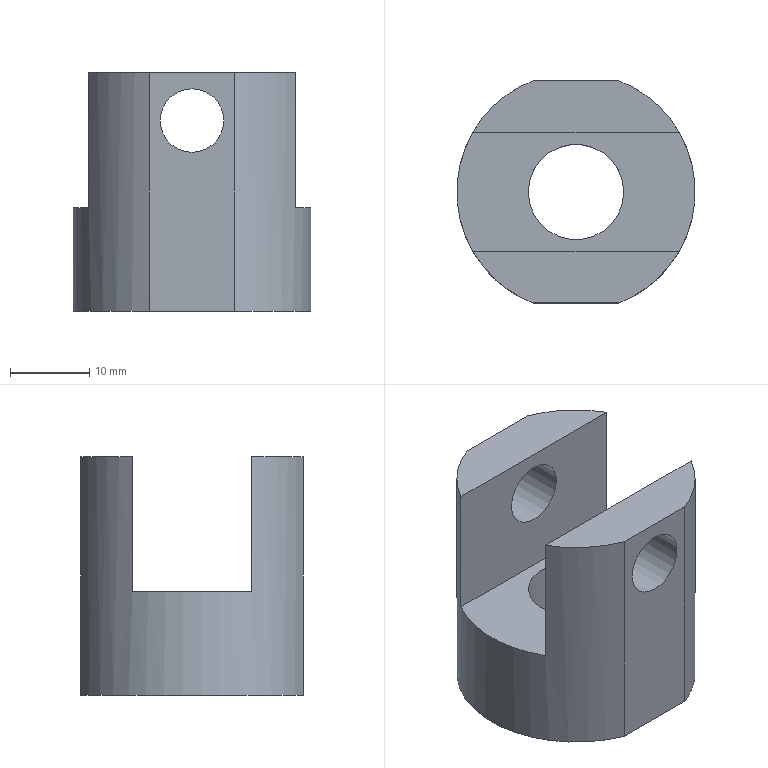Part | NX | features pneumatic support1 2 | 1 solid | 13 faces | box 30 x 28 x 30 mm | volume 11330 mm3 | plane 8 | cylinder 5 | commonest cylinder face diameters 8 x2 30 x2 12 x1
STEP:
#1=CARTESIAN_POINT('',(0.,-7.5,28.));
#2=VERTEX_POINT('',#1);
#3=CARTESIAN_POINT('',(0.,-7.5,24.));
#4=DIRECTION('',(0.,1.,0.));
#5=DIRECTION('',(0.,0.,1.));
#6=AXIS2_PLACEMENT_3D('',#3,#4,#5);
#7=CIRCLE('',#6,4.);
#8=EDGE_CURVE('',#2,#2,#7,.T.);
#9=ORIENTED_EDGE('',*,*,#8,.T.);
#10=EDGE_LOOP('',(#9));
#11=FACE_BOUND('',#10,.T.);
#12=CARTESIAN_POINT('',(0.,-14.,28.));
#13=VERTEX_POINT('',#12);
#14=CARTESIAN_POINT('',(0.,-14.,24.));
#15=DIRECTION('',(0.,1.,0.));
#16=DIRECTION('',(0.,0.,1.));
#17=AXIS2_PLACEMENT_3D('',#14,#15,#16);
#18=CIRCLE('',#17,4.);
#19=EDGE_CURVE('',#13,#13,#18,.T.);
#20=ORIENTED_EDGE('',*,*,#19,.F.);
#21=EDGE_LOOP('',(#20));
#22=FACE_BOUND('',#21,.T.);
#23=CARTESIAN_POINT('',(0.,-20.,24.));
#24=DIRECTION('',(0.,1.,0.));
#25=DIRECTION('',(0.,0.,1.));
#26=AXIS2_PLACEMENT_3D('',#23,#24,#25);
#27=CYLINDRICAL_SURFACE('',#26,4.);
#28=ADVANCED_FACE('',(#11,#22),#27,.F.);
#29=CARTESIAN_POINT('',(-6.,0.,13.));
#30=VERTEX_POINT('',#29);
#31=CARTESIAN_POINT('',(0.,0.,13.));
#32=DIRECTION('',(0.,0.,-1.));
#33=DIRECTION('',(-1.,0.,0.));
#34=AXIS2_PLACEMENT_3D('',#31,#32,#33);
#35=CIRCLE('',#34,6.);
#36=EDGE_CURVE('',#30,#30,#35,.T.);
#37=ORIENTED_EDGE('',*,*,#36,.F.);
#38=EDGE_LOOP('',(#37));
#39=FACE_BOUND('',#38,.T.);
#40=CARTESIAN_POINT('',(-6.,0.,0.));
#41=VERTEX_POINT('',#40);
#42=CARTESIAN_POINT('',(0.,0.,0.));
#43=DIRECTION('',(0.,0.,-1.));
#44=DIRECTION('',(-1.,0.,0.));
#45=AXIS2_PLACEMENT_3D('',#42,#43,#44);
#46=CIRCLE('',#45,6.);
#47=EDGE_CURVE('',#41,#41,#46,.T.);
#48=ORIENTED_EDGE('',*,*,#47,.T.);
#49=EDGE_LOOP('',(#48));
#50=FACE_BOUND('',#49,.T.);
#51=CARTESIAN_POINT('',(0.,0.,0.));
#52=DIRECTION('',(0.,0.,-1.));
#53=DIRECTION('',(-1.,0.,0.));
#54=AXIS2_PLACEMENT_3D('',#51,#52,#53);
#55=CYLINDRICAL_SURFACE('',#54,6.);
#56=ADVANCED_FACE('',(#39,#50),#55,.F.);
#57=CARTESIAN_POINT('',(0.,7.5,28.));
#58=VERTEX_POINT('',#57);
#59=CARTESIAN_POINT('',(0.,7.5,24.));
#60=DIRECTION('',(0.,1.,0.));
#61=DIRECTION('',(0.,0.,1.));
#62=AXIS2_PLACEMENT_3D('',#59,#60,#61);
#63=CIRCLE('',#62,4.);
#64=EDGE_CURVE('',#58,#58,#63,.F.);
#65=ORIENTED_EDGE('',*,*,#64,.T.);
#66=EDGE_LOOP('',(#65));
#67=FACE_BOUND('',#66,.T.);
#68=CARTESIAN_POINT('',(0.,14.,28.));
#69=VERTEX_POINT('',#68);
#70=CARTESIAN_POINT('',(0.,14.,24.));
#71=DIRECTION('',(0.,1.,0.));
#72=DIRECTION('',(0.,0.,1.));
#73=AXIS2_PLACEMENT_3D('',#70,#71,#72);
#74=CIRCLE('',#73,4.);
#75=EDGE_CURVE('',#69,#69,#74,.F.);
#76=ORIENTED_EDGE('',*,*,#75,.F.);
#77=EDGE_LOOP('',(#76));
#78=FACE_BOUND('',#77,.T.);
#79=CARTESIAN_POINT('',(0.,-20.,24.));
#80=DIRECTION('',(0.,1.,0.));
#81=DIRECTION('',(0.,0.,1.));
#82=AXIS2_PLACEMENT_3D('',#79,#80,#81);
#83=CYLINDRICAL_SURFACE('',#82,4.);
#84=ADVANCED_FACE('',(#67,#78),#83,.F.);
#85=CARTESIAN_POINT('',(-5.385,14.,0.));
#86=VERTEX_POINT('',#85);
#87=CARTESIAN_POINT('',(-5.385,14.,30.));
#88=VERTEX_POINT('',#87);
#89=CARTESIAN_POINT('',(-5.385,14.,30.));
#90=DIRECTION('',(0.,0.,1.));
#91=VECTOR('',#90,1000.);
#92=LINE('',#89,#91);
#93=EDGE_CURVE('',#86,#88,#92,.T.);
#94=ORIENTED_EDGE('',*,*,#93,.F.);
#95=CARTESIAN_POINT('',(-5.385,-14.,0.));
#96=VERTEX_POINT('',#95);
#97=CARTESIAN_POINT('',(0.,0.,0.));
#98=DIRECTION('',(0.,0.,-1.));
#99=DIRECTION('',(-1.,0.,0.));
#100=AXIS2_PLACEMENT_3D('',#97,#98,#99);
#101=CIRCLE('',#100,15.);
#102=EDGE_CURVE('',#86,#96,#101,.F.);
#103=ORIENTED_EDGE('',*,*,#102,.T.);
#104=CARTESIAN_POINT('',(-5.385,-14.,30.));
#105=VERTEX_POINT('',#104);
#106=CARTESIAN_POINT('',(-5.385,-14.,30.));
#107=DIRECTION('',(0.,0.,-1.));
#108=VECTOR('',#107,1000.);
#109=LINE('',#106,#108);
#110=EDGE_CURVE('',#105,#96,#109,.T.);
#111=ORIENTED_EDGE('',*,*,#110,.F.);
#112=CARTESIAN_POINT('',(-12.99,-7.5,30.));
#113=VERTEX_POINT('',#112);
#114=CARTESIAN_POINT('',(0.,0.,30.));
#115=DIRECTION('',(0.,0.,-1.));
#116=DIRECTION('',(-1.,0.,0.));
#117=AXIS2_PLACEMENT_3D('',#114,#115,#116);
#118=CIRCLE('',#117,15.);
#119=EDGE_CURVE('',#113,#105,#118,.F.);
#120=ORIENTED_EDGE('',*,*,#119,.F.);
#121=CARTESIAN_POINT('',(-12.99,-7.5,13.));
#122=VERTEX_POINT('',#121);
#123=CARTESIAN_POINT('',(-12.99,-7.5,13.));
#124=DIRECTION('',(0.,0.,-1.));
#125=VECTOR('',#124,1000.);
#126=LINE('',#123,#125);
#127=EDGE_CURVE('',#113,#122,#126,.T.);
#128=ORIENTED_EDGE('',*,*,#127,.T.);
#129=CARTESIAN_POINT('',(-12.99,7.5,13.));
#130=VERTEX_POINT('',#129);
#131=CARTESIAN_POINT('',(0.,0.,13.));
#132=DIRECTION('',(0.,0.,-1.));
#133=DIRECTION('',(-1.,0.,0.));
#134=AXIS2_PLACEMENT_3D('',#131,#132,#133);
#135=CIRCLE('',#134,15.);
#136=EDGE_CURVE('',#130,#122,#135,.F.);
#137=ORIENTED_EDGE('',*,*,#136,.F.);
#138=CARTESIAN_POINT('',(-12.99,7.5,30.));
#139=VERTEX_POINT('',#138);
#140=CARTESIAN_POINT('',(-12.99,7.5,13.));
#141=DIRECTION('',(0.,0.,1.));
#142=VECTOR('',#141,1000.);
#143=LINE('',#140,#142);
#144=EDGE_CURVE('',#130,#139,#143,.T.);
#145=ORIENTED_EDGE('',*,*,#144,.T.);
#146=CARTESIAN_POINT('',(0.,0.,30.));
#147=DIRECTION('',(0.,0.,-1.));
#148=DIRECTION('',(-1.,0.,0.));
#149=AXIS2_PLACEMENT_3D('',#146,#147,#148);
#150=CIRCLE('',#149,15.);
#151=EDGE_CURVE('',#88,#139,#150,.F.);
#152=ORIENTED_EDGE('',*,*,#151,.F.);
#153=EDGE_LOOP('',(#94,#103,#111,#120,#128,#137,#145,#152));
#154=FACE_BOUND('',#153,.T.);
#155=CARTESIAN_POINT('',(0.,0.,30.));
#156=DIRECTION('',(0.,0.,-1.));
#157=DIRECTION('',(-1.,0.,0.));
#158=AXIS2_PLACEMENT_3D('',#155,#156,#157);
#159=CYLINDRICAL_SURFACE('',#158,15.);
#160=ADVANCED_FACE('',(#154),#159,.T.);
#161=ORIENTED_EDGE('',*,*,#144,.F.);
#162=CARTESIAN_POINT('',(12.99,7.5,13.));
#163=VERTEX_POINT('',#162);
#164=CARTESIAN_POINT('',(-15.,7.5,13.));
#165=DIRECTION('',(1.,0.,0.));
#166=VECTOR('',#165,1000.);
#167=LINE('',#164,#166);
#168=EDGE_CURVE('',#163,#130,#167,.F.);
#169=ORIENTED_EDGE('',*,*,#168,.F.);
#170=CARTESIAN_POINT('',(12.99,7.5,30.));
#171=VERTEX_POINT('',#170);
#172=CARTESIAN_POINT('',(12.99,7.5,30.));
#173=DIRECTION('',(0.,0.,-1.));
#174=VECTOR('',#173,1000.);
#175=LINE('',#172,#174);
#176=EDGE_CURVE('',#171,#163,#175,.T.);
#177=ORIENTED_EDGE('',*,*,#176,.F.);
#178=CARTESIAN_POINT('',(0.,7.5,30.));
#179=DIRECTION('',(1.,0.,0.));
#180=VECTOR('',#179,1000.);
#181=LINE('',#178,#180);
#182=EDGE_CURVE('',#139,#171,#181,.T.);
#183=ORIENTED_EDGE('',*,*,#182,.F.);
#184=EDGE_LOOP('',(#161,#169,#177,#183));
#185=FACE_BOUND('',#184,.T.);
#186=ORIENTED_EDGE('',*,*,#64,.F.);
#187=EDGE_LOOP('',(#186));
#188=FACE_BOUND('',#187,.T.);
#189=CARTESIAN_POINT('',(15.,7.5,13.));
#190=DIRECTION('',(0.,1.,0.));
#191=DIRECTION('',(0.,0.,1.));
#192=AXIS2_PLACEMENT_3D('',#189,#190,#191);
#193=PLANE('',#192);
#194=ADVANCED_FACE('',(#185,#188),#193,.F.);
#195=CARTESIAN_POINT('',(12.99,-7.5,13.));
#196=VERTEX_POINT('',#195);
#197=CARTESIAN_POINT('',(15.,-7.5,13.));
#198=DIRECTION('',(1.,0.,0.));
#199=VECTOR('',#198,1000.);
#200=LINE('',#197,#199);
#201=EDGE_CURVE('',#122,#196,#200,.T.);
#202=ORIENTED_EDGE('',*,*,#201,.T.);
#203=CARTESIAN_POINT('',(0.,0.,13.));
#204=DIRECTION('',(0.,0.,-1.));
#205=DIRECTION('',(-1.,0.,0.));
#206=AXIS2_PLACEMENT_3D('',#203,#204,#205);
#207=CIRCLE('',#206,15.);
#208=EDGE_CURVE('',#163,#196,#207,.T.);
#209=ORIENTED_EDGE('',*,*,#208,.F.);
#210=ORIENTED_EDGE('',*,*,#168,.T.);
#211=ORIENTED_EDGE('',*,*,#136,.T.);
#212=EDGE_LOOP('',(#202,#209,#210,#211));
#213=FACE_BOUND('',#212,.T.);
#214=ORIENTED_EDGE('',*,*,#36,.T.);
#215=EDGE_LOOP('',(#214));
#216=FACE_BOUND('',#215,.T.);
#217=CARTESIAN_POINT('',(-15.,7.5,13.));
#218=DIRECTION('',(0.,0.,1.));
#219=DIRECTION('',(1.,0.,0.));
#220=AXIS2_PLACEMENT_3D('',#217,#218,#219);
#221=PLANE('',#220);
#222=ADVANCED_FACE('',(#213,#216),#221,.T.);
#223=CARTESIAN_POINT('',(12.99,-7.5,30.));
#224=VERTEX_POINT('',#223);
#225=CARTESIAN_POINT('',(12.99,-7.5,30.));
#226=DIRECTION('',(0.,0.,-1.));
#227=VECTOR('',#226,1000.);
#228=LINE('',#225,#227);
#229=EDGE_CURVE('',#196,#224,#228,.F.);
#230=ORIENTED_EDGE('',*,*,#229,.F.);
#231=ORIENTED_EDGE('',*,*,#201,.F.);
#232=ORIENTED_EDGE('',*,*,#127,.F.);
#233=CARTESIAN_POINT('',(0.,-7.5,30.));
#234=DIRECTION('',(1.,0.,0.));
#235=VECTOR('',#234,1000.);
#236=LINE('',#233,#235);
#237=EDGE_CURVE('',#224,#113,#236,.F.);
#238=ORIENTED_EDGE('',*,*,#237,.F.);
#239=EDGE_LOOP('',(#230,#231,#232,#238));
#240=FACE_BOUND('',#239,.T.);
#241=ORIENTED_EDGE('',*,*,#8,.F.);
#242=EDGE_LOOP('',(#241));
#243=FACE_BOUND('',#242,.T.);
#244=CARTESIAN_POINT('',(15.,-7.5,13.));
#245=DIRECTION('',(0.,-1.,0.));
#246=DIRECTION('',(0.,0.,-1.));
#247=AXIS2_PLACEMENT_3D('',#244,#245,#246);
#248=PLANE('',#247);
#249=ADVANCED_FACE('',(#240,#243),#248,.F.);
#250=CARTESIAN_POINT('',(5.385,-14.,30.));
#251=VERTEX_POINT('',#250);
#252=CARTESIAN_POINT('',(0.,0.,30.));
#253=DIRECTION('',(0.,0.,-1.));
#254=DIRECTION('',(-1.,0.,0.));
#255=AXIS2_PLACEMENT_3D('',#252,#253,#254);
#256=CIRCLE('',#255,15.);
#257=EDGE_CURVE('',#224,#251,#256,.T.);
#258=ORIENTED_EDGE('',*,*,#257,.F.);
#259=ORIENTED_EDGE('',*,*,#237,.T.);
#260=ORIENTED_EDGE('',*,*,#119,.T.);
#261=CARTESIAN_POINT('',(15.,-14.,30.));
#262=DIRECTION('',(1.,0.,0.));
#263=VECTOR('',#262,1000.);
#264=LINE('',#261,#263);
#265=EDGE_CURVE('',#251,#105,#264,.F.);
#266=ORIENTED_EDGE('',*,*,#265,.F.);
#267=EDGE_LOOP('',(#258,#259,#260,#266));
#268=FACE_BOUND('',#267,.T.);
#269=CARTESIAN_POINT('',(0.,0.,30.));
#270=DIRECTION('',(0.,0.,1.));
#271=DIRECTION('',(1.,0.,0.));
#272=AXIS2_PLACEMENT_3D('',#269,#270,#271);
#273=PLANE('',#272);
#274=ADVANCED_FACE('',(#268),#273,.T.);
#275=CARTESIAN_POINT('',(5.385,-14.,0.));
#276=VERTEX_POINT('',#275);
#277=CARTESIAN_POINT('',(5.385,-14.,30.));
#278=DIRECTION('',(0.,0.,-1.));
#279=VECTOR('',#278,1000.);
#280=LINE('',#277,#279);
#281=EDGE_CURVE('',#251,#276,#280,.T.);
#282=ORIENTED_EDGE('',*,*,#281,.F.);
#283=ORIENTED_EDGE('',*,*,#265,.T.);
#284=ORIENTED_EDGE('',*,*,#110,.T.);
#285=CARTESIAN_POINT('',(0.,-14.,0.));
#286=DIRECTION('',(1.,0.,0.));
#287=VECTOR('',#286,1000.);
#288=LINE('',#285,#287);
#289=EDGE_CURVE('',#96,#276,#288,.T.);
#290=ORIENTED_EDGE('',*,*,#289,.T.);
#291=EDGE_LOOP('',(#282,#283,#284,#290));
#292=FACE_BOUND('',#291,.T.);
#293=ORIENTED_EDGE('',*,*,#19,.T.);
#294=EDGE_LOOP('',(#293));
#295=FACE_BOUND('',#294,.T.);
#296=CARTESIAN_POINT('',(15.,-14.,30.));
#297=DIRECTION('',(0.,-1.,0.));
#298=DIRECTION('',(0.,0.,-1.));
#299=AXIS2_PLACEMENT_3D('',#296,#297,#298);
#300=PLANE('',#299);
#301=ADVANCED_FACE('',(#292,#295),#300,.T.);
#302=ORIENTED_EDGE('',*,*,#102,.F.);
#303=CARTESIAN_POINT('',(5.385,14.,0.));
#304=VERTEX_POINT('',#303);
#305=CARTESIAN_POINT('',(15.,14.,0.));
#306=DIRECTION('',(1.,0.,0.));
#307=VECTOR('',#306,1000.);
#308=LINE('',#305,#307);
#309=EDGE_CURVE('',#304,#86,#308,.F.);
#310=ORIENTED_EDGE('',*,*,#309,.F.);
#311=CARTESIAN_POINT('',(0.,0.,0.));
#312=DIRECTION('',(0.,0.,-1.));
#313=DIRECTION('',(-1.,0.,0.));
#314=AXIS2_PLACEMENT_3D('',#311,#312,#313);
#315=CIRCLE('',#314,15.);
#316=EDGE_CURVE('',#276,#304,#315,.F.);
#317=ORIENTED_EDGE('',*,*,#316,.F.);
#318=ORIENTED_EDGE('',*,*,#289,.F.);
#319=EDGE_LOOP('',(#302,#310,#317,#318));
#320=FACE_BOUND('',#319,.T.);
#321=ORIENTED_EDGE('',*,*,#47,.F.);
#322=EDGE_LOOP('',(#321));
#323=FACE_BOUND('',#322,.T.);
#324=CARTESIAN_POINT('',(0.,0.,0.));
#325=DIRECTION('',(0.,0.,1.));
#326=DIRECTION('',(1.,0.,0.));
#327=AXIS2_PLACEMENT_3D('',#324,#325,#326);
#328=PLANE('',#327);
#329=ADVANCED_FACE('',(#320,#323),#328,.F.);
#330=ORIENTED_EDGE('',*,*,#93,.T.);
#331=CARTESIAN_POINT('',(5.385,14.,30.));
#332=VERTEX_POINT('',#331);
#333=CARTESIAN_POINT('',(0.,14.,30.));
#334=DIRECTION('',(1.,0.,0.));
#335=VECTOR('',#334,1000.);
#336=LINE('',#333,#335);
#337=EDGE_CURVE('',#332,#88,#336,.F.);
#338=ORIENTED_EDGE('',*,*,#337,.F.);
#339=CARTESIAN_POINT('',(5.385,14.,30.));
#340=DIRECTION('',(0.,0.,-1.));
#341=VECTOR('',#340,1000.);
#342=LINE('',#339,#341);
#343=EDGE_CURVE('',#304,#332,#342,.F.);
#344=ORIENTED_EDGE('',*,*,#343,.F.);
#345=ORIENTED_EDGE('',*,*,#309,.T.);
#346=EDGE_LOOP('',(#330,#338,#344,#345));
#347=FACE_BOUND('',#346,.T.);
#348=ORIENTED_EDGE('',*,*,#75,.T.);
#349=EDGE_LOOP('',(#348));
#350=FACE_BOUND('',#349,.T.);
#351=CARTESIAN_POINT('',(15.,14.,30.));
#352=DIRECTION('',(0.,1.,0.));
#353=DIRECTION('',(0.,0.,1.));
#354=AXIS2_PLACEMENT_3D('',#351,#352,#353);
#355=PLANE('',#354);
#356=ADVANCED_FACE('',(#347,#350),#355,.T.);
#357=ORIENTED_EDGE('',*,*,#151,.T.);
#358=ORIENTED_EDGE('',*,*,#182,.T.);
#359=CARTESIAN_POINT('',(0.,0.,30.));
#360=DIRECTION('',(0.,0.,-1.));
#361=DIRECTION('',(-1.,0.,0.));
#362=AXIS2_PLACEMENT_3D('',#359,#360,#361);
#363=CIRCLE('',#362,15.);
#364=EDGE_CURVE('',#332,#171,#363,.T.);
#365=ORIENTED_EDGE('',*,*,#364,.F.);
#366=ORIENTED_EDGE('',*,*,#337,.T.);
#367=EDGE_LOOP('',(#357,#358,#365,#366));
#368=FACE_BOUND('',#367,.T.);
#369=CARTESIAN_POINT('',(0.,0.,30.));
#370=DIRECTION('',(0.,0.,1.));
#371=DIRECTION('',(1.,0.,0.));
#372=AXIS2_PLACEMENT_3D('',#369,#370,#371);
#373=PLANE('',#372);
#374=ADVANCED_FACE('',(#368),#373,.T.);
#375=ORIENTED_EDGE('',*,*,#343,.T.);
#376=ORIENTED_EDGE('',*,*,#364,.T.);
#377=ORIENTED_EDGE('',*,*,#176,.T.);
#378=ORIENTED_EDGE('',*,*,#208,.T.);
#379=ORIENTED_EDGE('',*,*,#229,.T.);
#380=ORIENTED_EDGE('',*,*,#257,.T.);
#381=ORIENTED_EDGE('',*,*,#281,.T.);
#382=ORIENTED_EDGE('',*,*,#316,.T.);
#383=EDGE_LOOP('',(#375,#376,#377,#378,#379,#380,#381,#382));
#384=FACE_BOUND('',#383,.T.);
#385=CARTESIAN_POINT('',(0.,0.,30.));
#386=DIRECTION('',(0.,0.,-1.));
#387=DIRECTION('',(-1.,0.,0.));
#388=AXIS2_PLACEMENT_3D('',#385,#386,#387);
#389=CYLINDRICAL_SURFACE('',#388,15.);
#390=ADVANCED_FACE('',(#384),#389,.T.);
#391=CLOSED_SHELL('',(#28,#56,#84,#160,#194,#222,#249,#274,#301,#329,#356,#374,#390));
#392=MANIFOLD_SOLID_BREP('',#391);
#393=(LENGTH_UNIT()NAMED_UNIT(*)SI_UNIT(.MILLI.,.METRE.));
#394=UNCERTAINTY_MEASURE_WITH_UNIT(LENGTH_MEASURE(0.00001),#393,'','');
#395=(NAMED_UNIT(*)PLANE_ANGLE_UNIT()SI_UNIT($,.RADIAN.));
#396=(NAMED_UNIT(*)SI_UNIT($,.STERADIAN.)SOLID_ANGLE_UNIT());
#397=(GEOMETRIC_REPRESENTATION_CONTEXT(3)GLOBAL_UNCERTAINTY_ASSIGNED_CONTEXT((#394))GLOBAL_UNIT_ASSIGNED_CONTEXT((#393,#395,#396))REPRESENTATION_CONTEXT('',''));
#398=ADVANCED_BREP_SHAPE_REPRESENTATION('',(#392),#397);